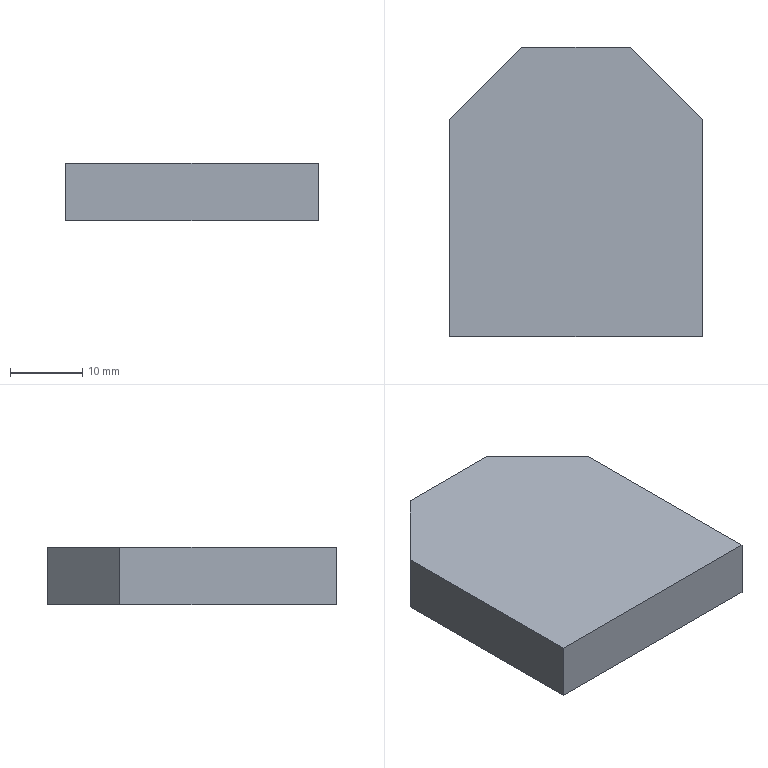Part | SolidWorks | features Extrusion 1 | 1 solid | 8 faces | box 35 x 40 x 8 mm | volume 10400 mm3 | plane 8
STEP:
#1=CARTESIAN_POINT('',(0.,30.,0.));
#2=VERTEX_POINT('',#1);
#3=CARTESIAN_POINT('',(0.,0.,0.));
#4=VERTEX_POINT('',#3);
#5=CARTESIAN_POINT('',(0.,0.,0.));
#6=DIRECTION('',(0.,-1.,0.));
#7=VECTOR('',#6,1000.);
#8=LINE('',#5,#7);
#9=EDGE_CURVE('',#2,#4,#8,.T.);
#10=ORIENTED_EDGE('',*,*,#9,.T.);
#11=CARTESIAN_POINT('',(0.,0.,8.));
#12=VERTEX_POINT('',#11);
#13=CARTESIAN_POINT('',(0.,0.,8.));
#14=DIRECTION('',(0.,0.,-1.));
#15=VECTOR('',#14,1000.);
#16=LINE('',#13,#15);
#17=EDGE_CURVE('',#12,#4,#16,.T.);
#18=ORIENTED_EDGE('',*,*,#17,.F.);
#19=CARTESIAN_POINT('',(0.,30.,8.));
#20=VERTEX_POINT('',#19);
#21=CARTESIAN_POINT('',(0.,0.,8.));
#22=DIRECTION('',(0.,-1.,0.));
#23=VECTOR('',#22,1000.);
#24=LINE('',#21,#23);
#25=EDGE_CURVE('',#20,#12,#24,.T.);
#26=ORIENTED_EDGE('',*,*,#25,.F.);
#27=CARTESIAN_POINT('',(0.,30.,8.));
#28=DIRECTION('',(0.,0.,-1.));
#29=VECTOR('',#28,1000.);
#30=LINE('',#27,#29);
#31=EDGE_CURVE('',#20,#2,#30,.T.);
#32=ORIENTED_EDGE('',*,*,#31,.T.);
#33=EDGE_LOOP('',(#10,#18,#26,#32));
#34=FACE_OUTER_BOUND('',#33,.T.);
#35=CARTESIAN_POINT('',(0.,0.,8.));
#36=DIRECTION('',(1.,0.,0.));
#37=DIRECTION('',(0.,0.,-1.));
#38=AXIS2_PLACEMENT_3D('',#35,#36,#37);
#39=PLANE('',#38);
#40=ADVANCED_FACE('',(#34),#39,.F.);
#41=CARTESIAN_POINT('',(35.,0.,0.));
#42=VERTEX_POINT('',#41);
#43=CARTESIAN_POINT('',(0.,0.,0.));
#44=DIRECTION('',(1.,0.,0.));
#45=VECTOR('',#44,1000.);
#46=LINE('',#43,#45);
#47=EDGE_CURVE('',#4,#42,#46,.T.);
#48=ORIENTED_EDGE('',*,*,#47,.T.);
#49=CARTESIAN_POINT('',(35.,0.,8.));
#50=VERTEX_POINT('',#49);
#51=CARTESIAN_POINT('',(35.,0.,8.));
#52=DIRECTION('',(0.,0.,-1.));
#53=VECTOR('',#52,1000.);
#54=LINE('',#51,#53);
#55=EDGE_CURVE('',#50,#42,#54,.T.);
#56=ORIENTED_EDGE('',*,*,#55,.F.);
#57=CARTESIAN_POINT('',(0.,0.,8.));
#58=DIRECTION('',(1.,0.,0.));
#59=VECTOR('',#58,1000.);
#60=LINE('',#57,#59);
#61=EDGE_CURVE('',#12,#50,#60,.T.);
#62=ORIENTED_EDGE('',*,*,#61,.F.);
#63=ORIENTED_EDGE('',*,*,#17,.T.);
#64=EDGE_LOOP('',(#48,#56,#62,#63));
#65=FACE_OUTER_BOUND('',#64,.T.);
#66=CARTESIAN_POINT('',(0.,0.,8.));
#67=DIRECTION('',(0.,1.,0.));
#68=DIRECTION('',(0.,0.,1.));
#69=AXIS2_PLACEMENT_3D('',#66,#67,#68);
#70=PLANE('',#69);
#71=ADVANCED_FACE('',(#65),#70,.F.);
#72=CARTESIAN_POINT('',(35.,30.,0.));
#73=VERTEX_POINT('',#72);
#74=CARTESIAN_POINT('',(35.,0.,0.));
#75=DIRECTION('',(0.,1.,0.));
#76=VECTOR('',#75,1000.);
#77=LINE('',#74,#76);
#78=EDGE_CURVE('',#42,#73,#77,.T.);
#79=ORIENTED_EDGE('',*,*,#78,.T.);
#80=CARTESIAN_POINT('',(35.,30.,8.));
#81=VERTEX_POINT('',#80);
#82=CARTESIAN_POINT('',(35.,30.,8.));
#83=DIRECTION('',(0.,0.,-1.));
#84=VECTOR('',#83,1000.);
#85=LINE('',#82,#84);
#86=EDGE_CURVE('',#81,#73,#85,.T.);
#87=ORIENTED_EDGE('',*,*,#86,.F.);
#88=CARTESIAN_POINT('',(35.,0.,8.));
#89=DIRECTION('',(0.,1.,0.));
#90=VECTOR('',#89,1000.);
#91=LINE('',#88,#90);
#92=EDGE_CURVE('',#50,#81,#91,.T.);
#93=ORIENTED_EDGE('',*,*,#92,.F.);
#94=ORIENTED_EDGE('',*,*,#55,.T.);
#95=EDGE_LOOP('',(#79,#87,#93,#94));
#96=FACE_OUTER_BOUND('',#95,.T.);
#97=CARTESIAN_POINT('',(35.,0.,8.));
#98=DIRECTION('',(-1.,0.,0.));
#99=DIRECTION('',(0.,0.,1.));
#100=AXIS2_PLACEMENT_3D('',#97,#98,#99);
#101=PLANE('',#100);
#102=ADVANCED_FACE('',(#96),#101,.F.);
#103=CARTESIAN_POINT('',(25.,40.,0.));
#104=VERTEX_POINT('',#103);
#105=CARTESIAN_POINT('',(25.,40.,0.));
#106=DIRECTION('',(-0.7071,0.7071,0.));
#107=VECTOR('',#106,1000.);
#108=LINE('',#105,#107);
#109=EDGE_CURVE('',#73,#104,#108,.T.);
#110=ORIENTED_EDGE('',*,*,#109,.T.);
#111=CARTESIAN_POINT('',(25.,40.,8.));
#112=VERTEX_POINT('',#111);
#113=CARTESIAN_POINT('',(25.,40.,8.));
#114=DIRECTION('',(0.,0.,-1.));
#115=VECTOR('',#114,1000.);
#116=LINE('',#113,#115);
#117=EDGE_CURVE('',#112,#104,#116,.T.);
#118=ORIENTED_EDGE('',*,*,#117,.F.);
#119=CARTESIAN_POINT('',(25.,40.,8.));
#120=DIRECTION('',(-0.7071,0.7071,0.));
#121=VECTOR('',#120,1000.);
#122=LINE('',#119,#121);
#123=EDGE_CURVE('',#81,#112,#122,.T.);
#124=ORIENTED_EDGE('',*,*,#123,.F.);
#125=ORIENTED_EDGE('',*,*,#86,.T.);
#126=EDGE_LOOP('',(#110,#118,#124,#125));
#127=FACE_OUTER_BOUND('',#126,.T.);
#128=CARTESIAN_POINT('',(25.,40.,8.));
#129=DIRECTION('',(-0.7071,-0.7071,0.));
#130=DIRECTION('',(0.7071,-0.7071,0.));
#131=AXIS2_PLACEMENT_3D('',#128,#129,#130);
#132=PLANE('',#131);
#133=ADVANCED_FACE('',(#127),#132,.F.);
#134=CARTESIAN_POINT('',(10.,40.,0.));
#135=VERTEX_POINT('',#134);
#136=CARTESIAN_POINT('',(10.,40.,0.));
#137=DIRECTION('',(-1.,0.,0.));
#138=VECTOR('',#137,1000.);
#139=LINE('',#136,#138);
#140=EDGE_CURVE('',#104,#135,#139,.T.);
#141=ORIENTED_EDGE('',*,*,#140,.T.);
#142=CARTESIAN_POINT('',(10.,40.,8.));
#143=VERTEX_POINT('',#142);
#144=CARTESIAN_POINT('',(10.,40.,8.));
#145=DIRECTION('',(0.,0.,-1.));
#146=VECTOR('',#145,1000.);
#147=LINE('',#144,#146);
#148=EDGE_CURVE('',#143,#135,#147,.T.);
#149=ORIENTED_EDGE('',*,*,#148,.F.);
#150=CARTESIAN_POINT('',(10.,40.,8.));
#151=DIRECTION('',(-1.,0.,0.));
#152=VECTOR('',#151,1000.);
#153=LINE('',#150,#152);
#154=EDGE_CURVE('',#112,#143,#153,.T.);
#155=ORIENTED_EDGE('',*,*,#154,.F.);
#156=ORIENTED_EDGE('',*,*,#117,.T.);
#157=EDGE_LOOP('',(#141,#149,#155,#156));
#158=FACE_OUTER_BOUND('',#157,.T.);
#159=CARTESIAN_POINT('',(10.,40.,8.));
#160=DIRECTION('',(0.,-1.,0.));
#161=DIRECTION('',(0.,0.,-1.));
#162=AXIS2_PLACEMENT_3D('',#159,#160,#161);
#163=PLANE('',#162);
#164=ADVANCED_FACE('',(#158),#163,.F.);
#165=CARTESIAN_POINT('',(0.,30.,0.));
#166=DIRECTION('',(-0.7071,-0.7071,0.));
#167=VECTOR('',#166,1000.);
#168=LINE('',#165,#167);
#169=EDGE_CURVE('',#135,#2,#168,.T.);
#170=ORIENTED_EDGE('',*,*,#169,.T.);
#171=ORIENTED_EDGE('',*,*,#31,.F.);
#172=CARTESIAN_POINT('',(0.,30.,8.));
#173=DIRECTION('',(-0.7071,-0.7071,0.));
#174=VECTOR('',#173,1000.);
#175=LINE('',#172,#174);
#176=EDGE_CURVE('',#143,#20,#175,.T.);
#177=ORIENTED_EDGE('',*,*,#176,.F.);
#178=ORIENTED_EDGE('',*,*,#148,.T.);
#179=EDGE_LOOP('',(#170,#171,#177,#178));
#180=FACE_OUTER_BOUND('',#179,.T.);
#181=CARTESIAN_POINT('',(0.,30.,8.));
#182=DIRECTION('',(0.7071,-0.7071,0.));
#183=DIRECTION('',(0.7071,0.7071,0.));
#184=AXIS2_PLACEMENT_3D('',#181,#182,#183);
#185=PLANE('',#184);
#186=ADVANCED_FACE('',(#180),#185,.F.);
#187=ORIENTED_EDGE('',*,*,#25,.T.);
#188=ORIENTED_EDGE('',*,*,#61,.T.);
#189=ORIENTED_EDGE('',*,*,#92,.T.);
#190=ORIENTED_EDGE('',*,*,#123,.T.);
#191=ORIENTED_EDGE('',*,*,#154,.T.);
#192=ORIENTED_EDGE('',*,*,#176,.T.);
#193=EDGE_LOOP('',(#187,#188,#189,#190,#191,#192));
#194=FACE_OUTER_BOUND('',#193,.T.);
#195=CARTESIAN_POINT('',(0.,0.,8.));
#196=DIRECTION('',(0.,0.,-1.));
#197=DIRECTION('',(-1.,0.,0.));
#198=AXIS2_PLACEMENT_3D('',#195,#196,#197);
#199=PLANE('',#198);
#200=ADVANCED_FACE('',(#194),#199,.F.);
#201=ORIENTED_EDGE('',*,*,#9,.F.);
#202=ORIENTED_EDGE('',*,*,#169,.F.);
#203=ORIENTED_EDGE('',*,*,#140,.F.);
#204=ORIENTED_EDGE('',*,*,#109,.F.);
#205=ORIENTED_EDGE('',*,*,#78,.F.);
#206=ORIENTED_EDGE('',*,*,#47,.F.);
#207=EDGE_LOOP('',(#201,#202,#203,#204,#205,#206));
#208=FACE_OUTER_BOUND('',#207,.T.);
#209=CARTESIAN_POINT('',(0.,0.,0.));
#210=DIRECTION('',(0.,0.,-1.));
#211=DIRECTION('',(-1.,0.,0.));
#212=AXIS2_PLACEMENT_3D('',#209,#210,#211);
#213=PLANE('',#212);
#214=ADVANCED_FACE('',(#208),#213,.T.);
#215=CLOSED_SHELL('',(#40,#71,#102,#133,#164,#186,#200,#214));
#216=MANIFOLD_SOLID_BREP('',#215);
#217=CARTESIAN_POINT('',(0.,0.,0.));
#218=DIRECTION('',(0.,0.,1.));
#219=DIRECTION('',(1.,0.,0.));
#220=AXIS2_PLACEMENT_3D('',#217,#218,#219);
#221=(LENGTH_UNIT()NAMED_UNIT(*)SI_UNIT(.MILLI.,.METRE.));
#222=UNCERTAINTY_MEASURE_WITH_UNIT(LENGTH_MEASURE(0.00001),#221,'','');
#223=(NAMED_UNIT(*)PLANE_ANGLE_UNIT()SI_UNIT($,.RADIAN.));
#224=(NAMED_UNIT(*)SI_UNIT($,.STERADIAN.)SOLID_ANGLE_UNIT());
#225=(GEOMETRIC_REPRESENTATION_CONTEXT(3)GLOBAL_UNCERTAINTY_ASSIGNED_CONTEXT((#222))GLOBAL_UNIT_ASSIGNED_CONTEXT((#221,#223,#224))REPRESENTATION_CONTEXT('',''));
#226=ADVANCED_BREP_SHAPE_REPRESENTATION('',(#216,#220),#225);